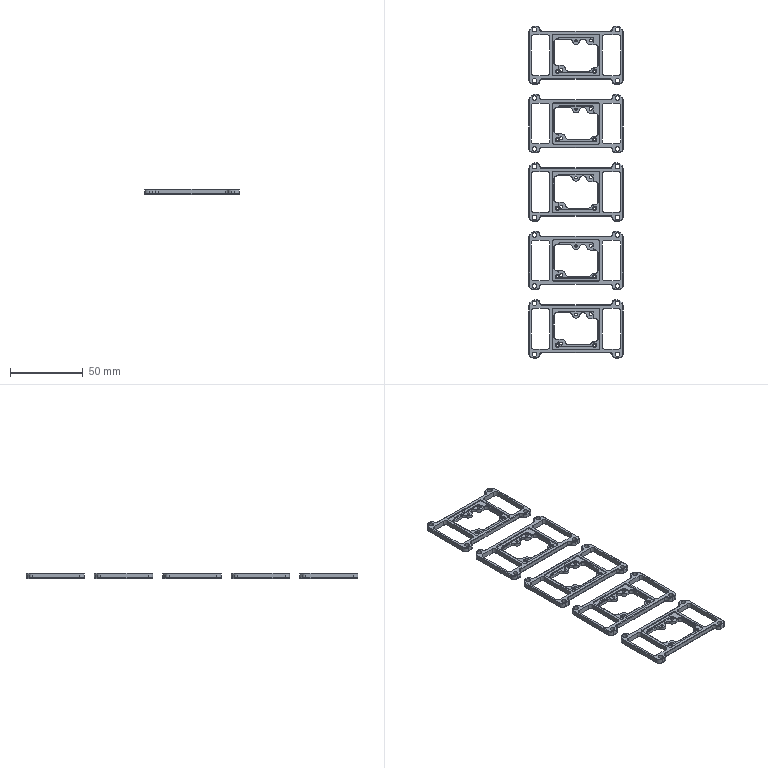NC program | NX | posted with a generic post | part box 65 x 228 x 3.5 mm
Lines 1 to 18 of 31259:
N10 G17 G21 G94 G90
(FLOOR_WALL , TOOL : D80)
N12 T19 M6
N14 G54
N16 G17 G0 G90 X159. Y0. S6500 M3
N18 G43 Z30. H19
N20 Z3.
N22 G94 G1 Z0. F1500.
N24 X156.
N26 X-156.
N28 X-159.
N30 Z3.
N32 G0 Z30.
N34 M5